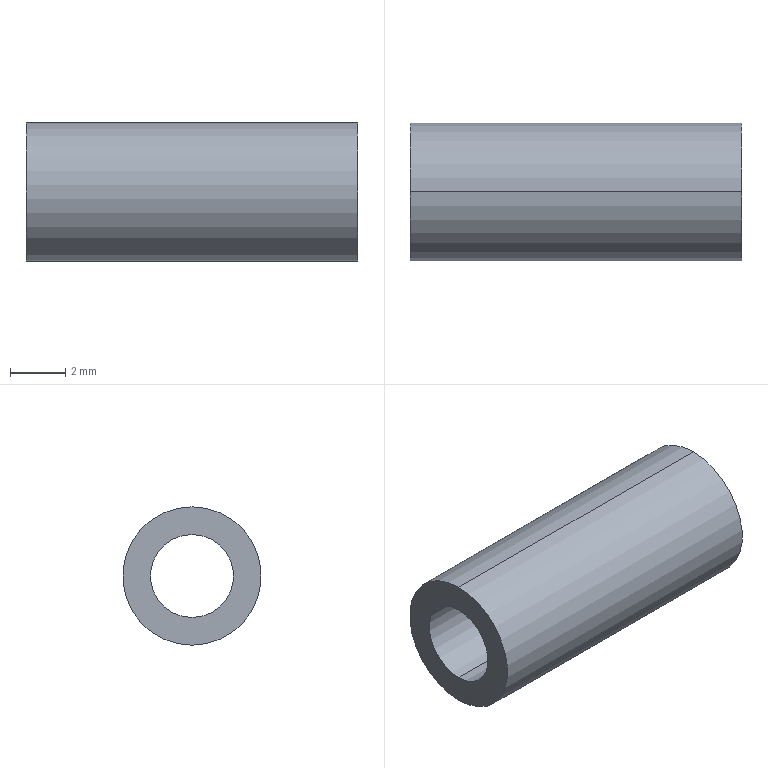Part | SolidWorks | features Extrusion 1 | 1 solid | 6 faces | box 12 x 5 x 5 mm | volume 150.796 mm3 | cylinder 4 | plane 2 | commonest cylinder face diameters 3 x2 5 x2
STEP:
#1=CARTESIAN_POINT('',(12.,0.,1.5));
#2=VERTEX_POINT('',#1);
#3=CARTESIAN_POINT('',(12.,0.,-1.5));
#4=VERTEX_POINT('',#3);
#5=CARTESIAN_POINT('',(12.,0.,0.));
#6=DIRECTION('',(1.,0.,0.));
#7=DIRECTION('',(0.,0.,-1.));
#8=AXIS2_PLACEMENT_3D('',#5,#6,#7);
#9=CIRCLE('',#8,1.5);
#10=EDGE_CURVE('',#2,#4,#9,.T.);
#11=ORIENTED_EDGE('',*,*,#10,.T.);
#12=CARTESIAN_POINT('',(0.,0.,-1.5));
#13=VERTEX_POINT('',#12);
#14=CARTESIAN_POINT('',(12.,0.,-1.5));
#15=DIRECTION('',(-1.,0.,0.));
#16=VECTOR('',#15,1000.);
#17=LINE('',#14,#16);
#18=EDGE_CURVE('',#4,#13,#17,.T.);
#19=ORIENTED_EDGE('',*,*,#18,.T.);
#20=CARTESIAN_POINT('',(0.,0.,1.5));
#21=VERTEX_POINT('',#20);
#22=CARTESIAN_POINT('',(0.,0.,0.));
#23=DIRECTION('',(1.,0.,0.));
#24=DIRECTION('',(0.,0.,-1.));
#25=AXIS2_PLACEMENT_3D('',#22,#23,#24);
#26=CIRCLE('',#25,1.5);
#27=EDGE_CURVE('',#21,#13,#26,.T.);
#28=ORIENTED_EDGE('',*,*,#27,.F.);
#29=CARTESIAN_POINT('',(12.,0.,1.5));
#30=DIRECTION('',(-1.,0.,0.));
#31=VECTOR('',#30,1000.);
#32=LINE('',#29,#31);
#33=EDGE_CURVE('',#2,#21,#32,.T.);
#34=ORIENTED_EDGE('',*,*,#33,.F.);
#35=EDGE_LOOP('',(#11,#19,#28,#34));
#36=FACE_OUTER_BOUND('',#35,.T.);
#37=CARTESIAN_POINT('',(12.,0.,0.));
#38=DIRECTION('',(-1.,0.,0.));
#39=DIRECTION('',(0.,0.,1.));
#40=AXIS2_PLACEMENT_3D('',#37,#38,#39);
#41=CYLINDRICAL_SURFACE('',#40,1.5);
#42=ADVANCED_FACE('',(#36),#41,.F.);
#43=CARTESIAN_POINT('',(12.,0.,-2.5));
#44=VERTEX_POINT('',#43);
#45=CARTESIAN_POINT('',(12.,0.,2.5));
#46=VERTEX_POINT('',#45);
#47=CARTESIAN_POINT('',(12.,0.,0.));
#48=DIRECTION('',(1.,0.,0.));
#49=DIRECTION('',(0.,0.,-1.));
#50=AXIS2_PLACEMENT_3D('',#47,#48,#49);
#51=CIRCLE('',#50,2.5);
#52=EDGE_CURVE('',#44,#46,#51,.T.);
#53=ORIENTED_EDGE('',*,*,#52,.F.);
#54=CARTESIAN_POINT('',(0.,0.,-2.5));
#55=VERTEX_POINT('',#54);
#56=CARTESIAN_POINT('',(12.,0.,-2.5));
#57=DIRECTION('',(-1.,0.,0.));
#58=VECTOR('',#57,1000.);
#59=LINE('',#56,#58);
#60=EDGE_CURVE('',#44,#55,#59,.T.);
#61=ORIENTED_EDGE('',*,*,#60,.T.);
#62=CARTESIAN_POINT('',(0.,0.,2.5));
#63=VERTEX_POINT('',#62);
#64=CARTESIAN_POINT('',(0.,0.,0.));
#65=DIRECTION('',(1.,0.,0.));
#66=DIRECTION('',(0.,0.,-1.));
#67=AXIS2_PLACEMENT_3D('',#64,#65,#66);
#68=CIRCLE('',#67,2.5);
#69=EDGE_CURVE('',#55,#63,#68,.T.);
#70=ORIENTED_EDGE('',*,*,#69,.T.);
#71=CARTESIAN_POINT('',(12.,0.,2.5));
#72=DIRECTION('',(-1.,0.,0.));
#73=VECTOR('',#72,1000.);
#74=LINE('',#71,#73);
#75=EDGE_CURVE('',#46,#63,#74,.T.);
#76=ORIENTED_EDGE('',*,*,#75,.F.);
#77=EDGE_LOOP('',(#53,#61,#70,#76));
#78=FACE_OUTER_BOUND('',#77,.T.);
#79=CARTESIAN_POINT('',(12.,0.,0.));
#80=DIRECTION('',(-1.,0.,0.));
#81=DIRECTION('',(0.,0.,1.));
#82=AXIS2_PLACEMENT_3D('',#79,#80,#81);
#83=CYLINDRICAL_SURFACE('',#82,2.5);
#84=ADVANCED_FACE('',(#78),#83,.T.);
#85=CARTESIAN_POINT('',(12.,0.,0.));
#86=DIRECTION('',(1.,0.,0.));
#87=DIRECTION('',(0.,0.,-1.));
#88=AXIS2_PLACEMENT_3D('',#85,#86,#87);
#89=CIRCLE('',#88,2.5);
#90=EDGE_CURVE('',#46,#44,#89,.T.);
#91=ORIENTED_EDGE('',*,*,#90,.T.);
#92=ORIENTED_EDGE('',*,*,#52,.T.);
#93=EDGE_LOOP('',(#91,#92));
#94=FACE_OUTER_BOUND('',#93,.T.);
#95=ORIENTED_EDGE('',*,*,#10,.F.);
#96=CARTESIAN_POINT('',(12.,0.,0.));
#97=DIRECTION('',(1.,0.,0.));
#98=DIRECTION('',(0.,0.,-1.));
#99=AXIS2_PLACEMENT_3D('',#96,#97,#98);
#100=CIRCLE('',#99,1.5);
#101=EDGE_CURVE('',#4,#2,#100,.T.);
#102=ORIENTED_EDGE('',*,*,#101,.F.);
#103=EDGE_LOOP('',(#95,#102));
#104=FACE_BOUND('',#103,.T.);
#105=CARTESIAN_POINT('',(12.,0.,0.));
#106=DIRECTION('',(1.,0.,0.));
#107=DIRECTION('',(0.,0.,-1.));
#108=AXIS2_PLACEMENT_3D('',#105,#106,#107);
#109=PLANE('',#108);
#110=ADVANCED_FACE('',(#94,#104),#109,.T.);
#111=CARTESIAN_POINT('',(0.,0.,0.));
#112=DIRECTION('',(1.,0.,0.));
#113=DIRECTION('',(0.,0.,-1.));
#114=AXIS2_PLACEMENT_3D('',#111,#112,#113);
#115=CIRCLE('',#114,2.5);
#116=EDGE_CURVE('',#63,#55,#115,.T.);
#117=ORIENTED_EDGE('',*,*,#116,.F.);
#118=ORIENTED_EDGE('',*,*,#69,.F.);
#119=EDGE_LOOP('',(#117,#118));
#120=FACE_OUTER_BOUND('',#119,.T.);
#121=ORIENTED_EDGE('',*,*,#27,.T.);
#122=CARTESIAN_POINT('',(0.,0.,0.));
#123=DIRECTION('',(1.,0.,0.));
#124=DIRECTION('',(0.,0.,-1.));
#125=AXIS2_PLACEMENT_3D('',#122,#123,#124);
#126=CIRCLE('',#125,1.5);
#127=EDGE_CURVE('',#13,#21,#126,.T.);
#128=ORIENTED_EDGE('',*,*,#127,.T.);
#129=EDGE_LOOP('',(#121,#128));
#130=FACE_BOUND('',#129,.T.);
#131=CARTESIAN_POINT('',(0.,0.,0.));
#132=DIRECTION('',(1.,0.,0.));
#133=DIRECTION('',(0.,0.,-1.));
#134=AXIS2_PLACEMENT_3D('',#131,#132,#133);
#135=PLANE('',#134);
#136=ADVANCED_FACE('',(#120,#130),#135,.F.);
#137=ORIENTED_EDGE('',*,*,#60,.F.);
#138=ORIENTED_EDGE('',*,*,#90,.F.);
#139=ORIENTED_EDGE('',*,*,#75,.T.);
#140=ORIENTED_EDGE('',*,*,#116,.T.);
#141=EDGE_LOOP('',(#137,#138,#139,#140));
#142=FACE_OUTER_BOUND('',#141,.T.);
#143=CARTESIAN_POINT('',(12.,0.,0.));
#144=DIRECTION('',(-1.,0.,0.));
#145=DIRECTION('',(0.,0.,1.));
#146=AXIS2_PLACEMENT_3D('',#143,#144,#145);
#147=CYLINDRICAL_SURFACE('',#146,2.5);
#148=ADVANCED_FACE('',(#142),#147,.T.);
#149=ORIENTED_EDGE('',*,*,#18,.F.);
#150=ORIENTED_EDGE('',*,*,#101,.T.);
#151=ORIENTED_EDGE('',*,*,#33,.T.);
#152=ORIENTED_EDGE('',*,*,#127,.F.);
#153=EDGE_LOOP('',(#149,#150,#151,#152));
#154=FACE_OUTER_BOUND('',#153,.T.);
#155=CARTESIAN_POINT('',(12.,0.,0.));
#156=DIRECTION('',(-1.,0.,0.));
#157=DIRECTION('',(0.,0.,1.));
#158=AXIS2_PLACEMENT_3D('',#155,#156,#157);
#159=CYLINDRICAL_SURFACE('',#158,1.5);
#160=ADVANCED_FACE('',(#154),#159,.F.);
#161=CLOSED_SHELL('',(#42,#84,#110,#136,#148,#160));
#162=MANIFOLD_SOLID_BREP('',#161);
#163=CARTESIAN_POINT('',(0.,0.,0.));
#164=DIRECTION('',(0.,0.,1.));
#165=DIRECTION('',(1.,0.,0.));
#166=AXIS2_PLACEMENT_3D('',#163,#164,#165);
#167=(LENGTH_UNIT()NAMED_UNIT(*)SI_UNIT(.MILLI.,.METRE.));
#168=UNCERTAINTY_MEASURE_WITH_UNIT(LENGTH_MEASURE(0.00001),#167,'','');
#169=(NAMED_UNIT(*)PLANE_ANGLE_UNIT()SI_UNIT($,.RADIAN.));
#170=(NAMED_UNIT(*)SI_UNIT($,.STERADIAN.)SOLID_ANGLE_UNIT());
#171=(GEOMETRIC_REPRESENTATION_CONTEXT(3)GLOBAL_UNCERTAINTY_ASSIGNED_CONTEXT((#168))GLOBAL_UNIT_ASSIGNED_CONTEXT((#167,#169,#170))REPRESENTATION_CONTEXT('',''));
#172=ADVANCED_BREP_SHAPE_REPRESENTATION('',(#162,#166),#171);